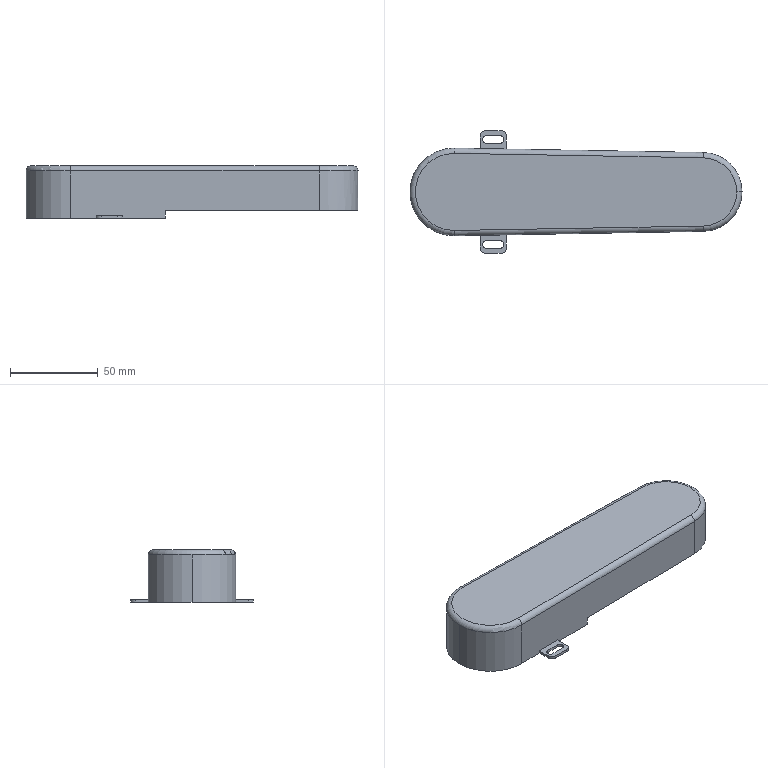Part | SolidWorks | features ICE 3, Extrusion 1, Fillet 1, MirrorPattern 1, Shell 1 | 1 solid | 48 faces | box 189.5 x 70 x 30 mm | volume 29758 mm3 | plane 22 | cylinder 20 | torus 6 | commonest cylinder face diameters 6 x8 4.2 x6 47 x2 50 x2 42 x1 45 x1
STEP:
#1=CARTESIAN_POINT('',(164.5,0.,27.));
#2=VERTEX_POINT('',#1);
#3=CARTESIAN_POINT('',(142.396,-22.497,27.));
#4=VERTEX_POINT('',#3);
#5=CARTESIAN_POINT('',(142.,0.,27.));
#6=DIRECTION('',(0.,0.,-1.));
#7=DIRECTION('',(1.,0.,0.));
#8=AXIS2_PLACEMENT_3D('',#5,#6,#7);
#9=CIRCLE('',#8,22.5);
#10=EDGE_CURVE('',#2,#4,#9,.T.);
#11=ORIENTED_EDGE('',*,*,#10,.F.);
#12=CARTESIAN_POINT('',(161.5,0.,30.));
#13=VERTEX_POINT('',#12);
#14=CARTESIAN_POINT('',(161.5,0.,27.));
#15=DIRECTION('',(0.,-1.,0.));
#16=DIRECTION('',(0.,0.,-1.));
#17=AXIS2_PLACEMENT_3D('',#14,#15,#16);
#18=CIRCLE('',#17,3.);
#19=EDGE_CURVE('',#2,#13,#18,.T.);
#20=ORIENTED_EDGE('',*,*,#19,.T.);
#21=CARTESIAN_POINT('',(142.343,-19.497,30.));
#22=VERTEX_POINT('',#21);
#23=CARTESIAN_POINT('',(142.,0.,30.));
#24=DIRECTION('',(0.,0.,1.));
#25=DIRECTION('',(1.,0.,0.));
#26=AXIS2_PLACEMENT_3D('',#23,#24,#25);
#27=CIRCLE('',#26,19.5);
#28=EDGE_CURVE('',#22,#13,#27,.T.);
#29=ORIENTED_EDGE('',*,*,#28,.F.);
#30=CARTESIAN_POINT('',(142.343,-19.497,27.));
#31=DIRECTION('',(-0.9998,-0.01761,0.));
#32=DIRECTION('',(0.01761,-0.9998,0.));
#33=AXIS2_PLACEMENT_3D('',#30,#31,#32);
#34=CIRCLE('',#33,3.);
#35=EDGE_CURVE('',#4,#22,#34,.T.);
#36=ORIENTED_EDGE('',*,*,#35,.F.);
#37=EDGE_LOOP('',(#11,#20,#29,#36));
#38=FACE_OUTER_BOUND('',#37,.T.);
#39=CARTESIAN_POINT('',(142.,0.,27.));
#40=DIRECTION('',(0.,0.,1.));
#41=DIRECTION('',(1.,0.,0.));
#42=AXIS2_PLACEMENT_3D('',#39,#40,#41);
#43=TOROIDAL_SURFACE('',#42,19.5,3.);
#44=ADVANCED_FACE('',(#38),#43,.T.);
#45=CARTESIAN_POINT('',(163.,0.,25.5));
#46=VERTEX_POINT('',#45);
#47=CARTESIAN_POINT('',(142.37,20.997,25.5));
#48=VERTEX_POINT('',#47);
#49=CARTESIAN_POINT('',(142.,0.,25.5));
#50=DIRECTION('',(0.,0.,1.));
#51=DIRECTION('',(1.,0.,0.));
#52=AXIS2_PLACEMENT_3D('',#49,#50,#51);
#53=CIRCLE('',#52,21.);
#54=EDGE_CURVE('',#46,#48,#53,.T.);
#55=ORIENTED_EDGE('',*,*,#54,.F.);
#56=CARTESIAN_POINT('',(160.,0.,28.5));
#57=VERTEX_POINT('',#56);
#58=CARTESIAN_POINT('',(160.,0.,25.5));
#59=DIRECTION('',(0.,-1.,0.));
#60=DIRECTION('',(0.,0.,-1.));
#61=AXIS2_PLACEMENT_3D('',#58,#59,#60);
#62=CIRCLE('',#61,3.);
#63=EDGE_CURVE('',#46,#57,#62,.T.);
#64=ORIENTED_EDGE('',*,*,#63,.T.);
#65=CARTESIAN_POINT('',(142.317,17.997,28.5));
#66=VERTEX_POINT('',#65);
#67=CARTESIAN_POINT('',(142.,0.,28.5));
#68=DIRECTION('',(0.,0.,-1.));
#69=DIRECTION('',(1.,0.,0.));
#70=AXIS2_PLACEMENT_3D('',#67,#68,#69);
#71=CIRCLE('',#70,18.);
#72=EDGE_CURVE('',#66,#57,#71,.T.);
#73=ORIENTED_EDGE('',*,*,#72,.F.);
#74=CARTESIAN_POINT('',(142.317,17.997,25.5));
#75=DIRECTION('',(-0.9998,0.01761,0.));
#76=DIRECTION('',(-0.01761,-0.9998,0.));
#77=AXIS2_PLACEMENT_3D('',#74,#75,#76);
#78=CIRCLE('',#77,3.);
#79=EDGE_CURVE('',#66,#48,#78,.T.);
#80=ORIENTED_EDGE('',*,*,#79,.T.);
#81=EDGE_LOOP('',(#55,#64,#73,#80));
#82=FACE_OUTER_BOUND('',#81,.T.);
#83=CARTESIAN_POINT('',(142.,0.,25.5));
#84=DIRECTION('',(0.,0.,1.));
#85=DIRECTION('',(1.,0.,0.));
#86=AXIS2_PLACEMENT_3D('',#83,#84,#85);
#87=TOROIDAL_SURFACE('',#86,18.,3.);
#88=ADVANCED_FACE('',(#82),#87,.F.);
#89=CARTESIAN_POINT('',(28.6,-30.,0.));
#90=VERTEX_POINT('',#89);
#91=CARTESIAN_POINT('',(26.5,-27.9,0.));
#92=VERTEX_POINT('',#91);
#93=CARTESIAN_POINT('',(26.5,-30.,0.));
#94=DIRECTION('',(0.,0.,1.));
#95=DIRECTION('',(1.,0.,0.));
#96=AXIS2_PLACEMENT_3D('',#93,#94,#95);
#97=CIRCLE('',#96,2.1);
#98=EDGE_CURVE('',#90,#92,#97,.T.);
#99=ORIENTED_EDGE('',*,*,#98,.F.);
#100=CARTESIAN_POINT('',(28.6,-30.,1.5));
#101=VERTEX_POINT('',#100);
#102=CARTESIAN_POINT('',(28.6,-30.,-12.903));
#103=DIRECTION('',(0.,0.,1.));
#104=VECTOR('',#103,1000.);
#105=LINE('',#102,#104);
#106=EDGE_CURVE('',#90,#101,#105,.T.);
#107=ORIENTED_EDGE('',*,*,#106,.T.);
#108=CARTESIAN_POINT('',(26.5,-27.9,1.5));
#109=VERTEX_POINT('',#108);
#110=CARTESIAN_POINT('',(26.5,-30.,1.5));
#111=DIRECTION('',(0.,0.,-1.));
#112=DIRECTION('',(1.,0.,0.));
#113=AXIS2_PLACEMENT_3D('',#110,#111,#112);
#114=CIRCLE('',#113,2.1);
#115=EDGE_CURVE('',#109,#101,#114,.T.);
#116=ORIENTED_EDGE('',*,*,#115,.F.);
#117=CARTESIAN_POINT('',(26.5,-27.9,-12.903));
#118=DIRECTION('',(0.,0.,1.));
#119=VECTOR('',#118,1000.);
#120=LINE('',#117,#119);
#121=EDGE_CURVE('',#92,#109,#120,.T.);
#122=ORIENTED_EDGE('',*,*,#121,.F.);
#123=EDGE_LOOP('',(#99,#107,#116,#122));
#124=FACE_OUTER_BOUND('',#123,.T.);
#125=CARTESIAN_POINT('',(26.5,-30.,-12.903));
#126=DIRECTION('',(0.,0.,1.));
#127=DIRECTION('',(1.,0.,0.));
#128=AXIS2_PLACEMENT_3D('',#125,#126,#127);
#129=CYLINDRICAL_SURFACE('',#128,2.1);
#130=ADVANCED_FACE('',(#124),#129,.F.);
#131=CARTESIAN_POINT('',(26.5,32.1,0.));
#132=VERTEX_POINT('',#131);
#133=CARTESIAN_POINT('',(28.6,30.,0.));
#134=VERTEX_POINT('',#133);
#135=CARTESIAN_POINT('',(26.5,30.,0.));
#136=DIRECTION('',(0.,0.,-1.));
#137=DIRECTION('',(1.,0.,0.));
#138=AXIS2_PLACEMENT_3D('',#135,#136,#137);
#139=CIRCLE('',#138,2.1);
#140=EDGE_CURVE('',#132,#134,#139,.T.);
#141=ORIENTED_EDGE('',*,*,#140,.T.);
#142=CARTESIAN_POINT('',(28.6,30.,1.5));
#143=VERTEX_POINT('',#142);
#144=CARTESIAN_POINT('',(28.6,30.,-12.903));
#145=DIRECTION('',(0.,0.,1.));
#146=VECTOR('',#145,1000.);
#147=LINE('',#144,#146);
#148=EDGE_CURVE('',#134,#143,#147,.T.);
#149=ORIENTED_EDGE('',*,*,#148,.T.);
#150=CARTESIAN_POINT('',(26.5,32.1,1.5));
#151=VERTEX_POINT('',#150);
#152=CARTESIAN_POINT('',(26.5,30.,1.5));
#153=DIRECTION('',(0.,0.,1.));
#154=DIRECTION('',(1.,0.,0.));
#155=AXIS2_PLACEMENT_3D('',#152,#153,#154);
#156=CIRCLE('',#155,2.1);
#157=EDGE_CURVE('',#143,#151,#156,.T.);
#158=ORIENTED_EDGE('',*,*,#157,.T.);
#159=CARTESIAN_POINT('',(26.5,32.1,-12.903));
#160=DIRECTION('',(0.,0.,1.));
#161=VECTOR('',#160,1000.);
#162=LINE('',#159,#161);
#163=EDGE_CURVE('',#132,#151,#162,.T.);
#164=ORIENTED_EDGE('',*,*,#163,.F.);
#165=EDGE_LOOP('',(#141,#149,#158,#164));
#166=FACE_OUTER_BOUND('',#165,.T.);
#167=CARTESIAN_POINT('',(26.5,30.,-12.903));
#168=DIRECTION('',(0.,0.,1.));
#169=DIRECTION('',(1.,0.,0.));
#170=AXIS2_PLACEMENT_3D('',#167,#168,#169);
#171=CYLINDRICAL_SURFACE('',#170,2.1);
#172=ADVANCED_FACE('',(#166),#171,.F.);
#173=CARTESIAN_POINT('',(0.4137,23.496,25.5));
#174=VERTEX_POINT('',#173);
#175=CARTESIAN_POINT('',(-23.5,0.,25.5));
#176=VERTEX_POINT('',#175);
#177=CARTESIAN_POINT('',(0.,0.,25.5));
#178=DIRECTION('',(0.,0.,1.));
#179=DIRECTION('',(1.,0.,0.));
#180=AXIS2_PLACEMENT_3D('',#177,#178,#179);
#181=CIRCLE('',#180,23.5);
#182=EDGE_CURVE('',#174,#176,#181,.T.);
#183=ORIENTED_EDGE('',*,*,#182,.T.);
#184=CARTESIAN_POINT('',(-23.5,0.,0.));
#185=VERTEX_POINT('',#184);
#186=CARTESIAN_POINT('',(-23.5,0.,30.));
#187=DIRECTION('',(0.,0.,-1.));
#188=VECTOR('',#187,1000.);
#189=LINE('',#186,#188);
#190=EDGE_CURVE('',#176,#185,#189,.T.);
#191=ORIENTED_EDGE('',*,*,#190,.T.);
#192=CARTESIAN_POINT('',(0.4137,23.496,0.));
#193=VERTEX_POINT('',#192);
#194=CARTESIAN_POINT('',(0.,0.,0.));
#195=DIRECTION('',(0.,0.,1.));
#196=DIRECTION('',(1.,0.,0.));
#197=AXIS2_PLACEMENT_3D('',#194,#195,#196);
#198=CIRCLE('',#197,23.5);
#199=EDGE_CURVE('',#193,#185,#198,.T.);
#200=ORIENTED_EDGE('',*,*,#199,.F.);
#201=CARTESIAN_POINT('',(0.4137,23.496,30.));
#202=DIRECTION('',(0.,0.,-1.));
#203=VECTOR('',#202,1000.);
#204=LINE('',#201,#203);
#205=EDGE_CURVE('',#174,#193,#204,.T.);
#206=ORIENTED_EDGE('',*,*,#205,.F.);
#207=EDGE_LOOP('',(#183,#191,#200,#206));
#208=FACE_OUTER_BOUND('',#207,.T.);
#209=CARTESIAN_POINT('',(0.,0.,30.));
#210=DIRECTION('',(0.,0.,-1.));
#211=DIRECTION('',(-1.,0.,0.));
#212=AXIS2_PLACEMENT_3D('',#209,#210,#211);
#213=CYLINDRICAL_SURFACE('',#212,23.5);
#214=ADVANCED_FACE('',(#208),#213,.F.);
#215=CARTESIAN_POINT('',(0.4401,-24.996,27.));
#216=VERTEX_POINT('',#215);
#217=CARTESIAN_POINT('',(-25.,0.,27.));
#218=VERTEX_POINT('',#217);
#219=CARTESIAN_POINT('',(0.,0.,27.));
#220=DIRECTION('',(0.,0.,-1.));
#221=DIRECTION('',(1.,0.,0.));
#222=AXIS2_PLACEMENT_3D('',#219,#220,#221);
#223=CIRCLE('',#222,25.);
#224=EDGE_CURVE('',#216,#218,#223,.T.);
#225=ORIENTED_EDGE('',*,*,#224,.T.);
#226=CARTESIAN_POINT('',(-25.,0.,0.));
#227=VERTEX_POINT('',#226);
#228=CARTESIAN_POINT('',(-25.,0.,30.));
#229=DIRECTION('',(0.,0.,-1.));
#230=VECTOR('',#229,1000.);
#231=LINE('',#228,#230);
#232=EDGE_CURVE('',#218,#227,#231,.T.);
#233=ORIENTED_EDGE('',*,*,#232,.T.);
#234=CARTESIAN_POINT('',(0.4401,-24.996,0.));
#235=VERTEX_POINT('',#234);
#236=CARTESIAN_POINT('',(0.,0.,0.));
#237=DIRECTION('',(0.,0.,1.));
#238=DIRECTION('',(1.,0.,0.));
#239=AXIS2_PLACEMENT_3D('',#236,#237,#238);
#240=CIRCLE('',#239,25.);
#241=EDGE_CURVE('',#227,#235,#240,.T.);
#242=ORIENTED_EDGE('',*,*,#241,.T.);
#243=CARTESIAN_POINT('',(0.4401,-24.996,30.));
#244=DIRECTION('',(0.,0.,-1.));
#245=VECTOR('',#244,1000.);
#246=LINE('',#243,#245);
#247=EDGE_CURVE('',#216,#235,#246,.T.);
#248=ORIENTED_EDGE('',*,*,#247,.F.);
#249=EDGE_LOOP('',(#225,#233,#242,#248));
#250=FACE_OUTER_BOUND('',#249,.T.);
#251=CARTESIAN_POINT('',(0.,0.,30.));
#252=DIRECTION('',(0.,0.,-1.));
#253=DIRECTION('',(-1.,0.,0.));
#254=AXIS2_PLACEMENT_3D('',#251,#252,#253);
#255=CYLINDRICAL_SURFACE('',#254,25.);
#256=ADVANCED_FACE('',(#250),#255,.T.);
#257=CARTESIAN_POINT('',(30.,-24.476,0.));
#258=VERTEX_POINT('',#257);
#259=CARTESIAN_POINT('',(54.5,-24.044,0.));
#260=VERTEX_POINT('',#259);
#261=CARTESIAN_POINT('',(0.4401,-24.996,0.));
#262=DIRECTION('',(0.9998,0.01761,0.));
#263=VECTOR('',#262,1000.);
#264=LINE('',#261,#263);
#265=EDGE_CURVE('',#258,#260,#264,.T.);
#266=ORIENTED_EDGE('',*,*,#265,.T.);
#267=CARTESIAN_POINT('',(54.5,-24.044,4.5));
#268=VERTEX_POINT('',#267);
#269=CARTESIAN_POINT('',(54.5,-24.044,30.));
#270=DIRECTION('',(0.,0.,1.));
#271=VECTOR('',#270,1000.);
#272=LINE('',#269,#271);
#273=EDGE_CURVE('',#260,#268,#272,.T.);
#274=ORIENTED_EDGE('',*,*,#273,.T.);
#275=CARTESIAN_POINT('',(142.396,-22.497,4.5));
#276=VERTEX_POINT('',#275);
#277=CARTESIAN_POINT('',(0.4401,-24.996,4.5));
#278=DIRECTION('',(0.9998,0.01761,0.));
#279=VECTOR('',#278,1000.);
#280=LINE('',#277,#279);
#281=EDGE_CURVE('',#268,#276,#280,.T.);
#282=ORIENTED_EDGE('',*,*,#281,.T.);
#283=CARTESIAN_POINT('',(142.396,-22.497,30.));
#284=DIRECTION('',(0.,0.,-1.));
#285=VECTOR('',#284,1000.);
#286=LINE('',#283,#285);
#287=EDGE_CURVE('',#4,#276,#286,.T.);
#288=ORIENTED_EDGE('',*,*,#287,.F.);
#289=CARTESIAN_POINT('',(0.4401,-24.996,27.));
#290=DIRECTION('',(-0.9998,-0.01761,0.));
#291=VECTOR('',#290,1000.);
#292=LINE('',#289,#291);
#293=EDGE_CURVE('',#4,#216,#292,.T.);
#294=ORIENTED_EDGE('',*,*,#293,.T.);
#295=ORIENTED_EDGE('',*,*,#247,.T.);
#296=CARTESIAN_POINT('',(15.,-24.74,0.));
#297=VERTEX_POINT('',#296);
#298=CARTESIAN_POINT('',(0.4401,-24.996,0.));
#299=DIRECTION('',(0.9998,0.01761,0.));
#300=VECTOR('',#299,1000.);
#301=LINE('',#298,#300);
#302=EDGE_CURVE('',#235,#297,#301,.T.);
#303=ORIENTED_EDGE('',*,*,#302,.T.);
#304=CARTESIAN_POINT('',(15.,-24.74,1.5));
#305=VERTEX_POINT('',#304);
#306=CARTESIAN_POINT('',(15.,-24.74,1.5));
#307=DIRECTION('',(0.,0.,-1.));
#308=VECTOR('',#307,1000.);
#309=LINE('',#306,#308);
#310=EDGE_CURVE('',#305,#297,#309,.T.);
#311=ORIENTED_EDGE('',*,*,#310,.F.);
#312=CARTESIAN_POINT('',(30.,-24.476,1.5));
#313=VERTEX_POINT('',#312);
#314=CARTESIAN_POINT('',(15.,-24.74,1.5));
#315=DIRECTION('',(-0.9998,-0.01761,0.));
#316=VECTOR('',#315,1000.);
#317=LINE('',#314,#316);
#318=EDGE_CURVE('',#313,#305,#317,.T.);
#319=ORIENTED_EDGE('',*,*,#318,.F.);
#320=CARTESIAN_POINT('',(30.,-24.476,1.5));
#321=DIRECTION('',(0.,0.,-1.));
#322=VECTOR('',#321,1000.);
#323=LINE('',#320,#322);
#324=EDGE_CURVE('',#313,#258,#323,.T.);
#325=ORIENTED_EDGE('',*,*,#324,.T.);
#326=EDGE_LOOP('',(#266,#274,#282,#288,#294,#295,#303,#311,#319,#325));
#327=FACE_OUTER_BOUND('',#326,.T.);
#328=CARTESIAN_POINT('',(0.4401,-24.996,30.));
#329=DIRECTION('',(-0.01761,0.9998,0.));
#330=DIRECTION('',(-0.9998,-0.01761,0.));
#331=AXIS2_PLACEMENT_3D('',#328,#329,#330);
#332=PLANE('',#331);
#333=ADVANCED_FACE('',(#327),#332,.F.);
#334=ORIENTED_EDGE('',*,*,#232,.F.);
#335=CARTESIAN_POINT('',(0.4401,24.996,27.));
#336=VERTEX_POINT('',#335);
#337=CARTESIAN_POINT('',(0.,0.,27.));
#338=DIRECTION('',(0.,0.,-1.));
#339=DIRECTION('',(1.,0.,0.));
#340=AXIS2_PLACEMENT_3D('',#337,#338,#339);
#341=CIRCLE('',#340,25.);
#342=EDGE_CURVE('',#218,#336,#341,.T.);
#343=ORIENTED_EDGE('',*,*,#342,.T.);
#344=CARTESIAN_POINT('',(0.4401,24.996,0.));
#345=VERTEX_POINT('',#344);
#346=CARTESIAN_POINT('',(0.4401,24.996,30.));
#347=DIRECTION('',(0.,0.,-1.));
#348=VECTOR('',#347,1000.);
#349=LINE('',#346,#348);
#350=EDGE_CURVE('',#336,#345,#349,.T.);
#351=ORIENTED_EDGE('',*,*,#350,.T.);
#352=CARTESIAN_POINT('',(0.,0.,0.));
#353=DIRECTION('',(0.,0.,1.));
#354=DIRECTION('',(1.,0.,0.));
#355=AXIS2_PLACEMENT_3D('',#352,#353,#354);
#356=CIRCLE('',#355,25.);
#357=EDGE_CURVE('',#345,#227,#356,.T.);
#358=ORIENTED_EDGE('',*,*,#357,.T.);
#359=EDGE_LOOP('',(#334,#343,#351,#358));
#360=FACE_OUTER_BOUND('',#359,.T.);
#361=CARTESIAN_POINT('',(0.,0.,30.));
#362=DIRECTION('',(0.,0.,-1.));
#363=DIRECTION('',(-1.,0.,0.));
#364=AXIS2_PLACEMENT_3D('',#361,#362,#363);
#365=CYLINDRICAL_SURFACE('',#364,25.);
#366=ADVANCED_FACE('',(#360),#365,.T.);
#367=CARTESIAN_POINT('',(142.396,22.497,4.5));
#368=VERTEX_POINT('',#367);
#369=CARTESIAN_POINT('',(142.,0.,4.5));
#370=DIRECTION('',(0.,0.,1.));
#371=DIRECTION('',(1.,0.,0.));
#372=AXIS2_PLACEMENT_3D('',#369,#370,#371);
#373=CIRCLE('',#372,22.5);
#374=EDGE_CURVE('',#276,#368,#373,.T.);
#375=ORIENTED_EDGE('',*,*,#374,.T.);
#376=CARTESIAN_POINT('',(142.396,22.497,27.));
#377=VERTEX_POINT('',#376);
#378=CARTESIAN_POINT('',(142.396,22.497,30.));
#379=DIRECTION('',(0.,0.,-1.));
#380=VECTOR('',#379,1000.);
#381=LINE('',#378,#380);
#382=EDGE_CURVE('',#377,#368,#381,.T.);
#383=ORIENTED_EDGE('',*,*,#382,.F.);
#384=CARTESIAN_POINT('',(142.,0.,27.));
#385=DIRECTION('',(0.,0.,-1.));
#386=DIRECTION('',(1.,0.,0.));
#387=AXIS2_PLACEMENT_3D('',#384,#385,#386);
#388=CIRCLE('',#387,22.5);
#389=EDGE_CURVE('',#377,#2,#388,.T.);
#390=ORIENTED_EDGE('',*,*,#389,.T.);
#391=ORIENTED_EDGE('',*,*,#10,.T.);
#392=ORIENTED_EDGE('',*,*,#287,.T.);
#393=EDGE_LOOP('',(#375,#383,#390,#391,#392));
#394=FACE_OUTER_BOUND('',#393,.T.);
#395=CARTESIAN_POINT('',(142.,0.,30.));
#396=DIRECTION('',(0.,0.,-1.));
#397=DIRECTION('',(-1.,0.,0.));
#398=AXIS2_PLACEMENT_3D('',#395,#396,#397);
#399=CYLINDRICAL_SURFACE('',#398,22.5);
#400=ADVANCED_FACE('',(#394),#399,.T.);
#401=CARTESIAN_POINT('',(54.5,24.044,4.5));
#402=VERTEX_POINT('',#401);
#403=CARTESIAN_POINT('',(0.4401,24.996,4.5));
#404=DIRECTION('',(-0.9998,0.01761,0.));
#405=VECTOR('',#404,1000.);
#406=LINE('',#403,#405);
#407=EDGE_CURVE('',#368,#402,#406,.T.);
#408=ORIENTED_EDGE('',*,*,#407,.T.);
#409=CARTESIAN_POINT('',(54.5,24.044,0.));
#410=VERTEX_POINT('',#409);
#411=CARTESIAN_POINT('',(54.5,24.044,30.));
#412=DIRECTION('',(0.,0.,-1.));
#413=VECTOR('',#412,1000.);
#414=LINE('',#411,#413);
#415=EDGE_CURVE('',#402,#410,#414,.T.);
#416=ORIENTED_EDGE('',*,*,#415,.T.);
#417=CARTESIAN_POINT('',(30.,24.476,0.));
#418=VERTEX_POINT('',#417);
#419=CARTESIAN_POINT('',(0.4401,24.996,0.));
#420=DIRECTION('',(-0.9998,0.01761,0.));
#421=VECTOR('',#420,1000.);
#422=LINE('',#419,#421);
#423=EDGE_CURVE('',#410,#418,#422,.T.);
#424=ORIENTED_EDGE('',*,*,#423,.T.);
#425=CARTESIAN_POINT('',(30.,24.476,1.5));
#426=VERTEX_POINT('',#425);
#427=CARTESIAN_POINT('',(30.,24.476,1.5));
#428=DIRECTION('',(0.,0.,-1.));
#429=VECTOR('',#428,1000.);
#430=LINE('',#427,#429);
#431=EDGE_CURVE('',#426,#418,#430,.T.);
#432=ORIENTED_EDGE('',*,*,#431,.F.);
#433=CARTESIAN_POINT('',(15.,24.74,1.5));
#434=VERTEX_POINT('',#433);
#435=CARTESIAN_POINT('',(15.,24.74,1.5));
#436=DIRECTION('',(-0.9998,0.01761,0.));
#437=VECTOR('',#436,1000.);
#438=LINE('',#435,#437);
#439=EDGE_CURVE('',#426,#434,#438,.T.);
#440=ORIENTED_EDGE('',*,*,#439,.T.);
#441=CARTESIAN_POINT('',(15.,24.74,0.));
#442=VERTEX_POINT('',#441);
#443=CARTESIAN_POINT('',(15.,24.74,1.5));
#444=DIRECTION('',(0.,0.,-1.));
#445=VECTOR('',#444,1000.);
#446=LINE('',#443,#445);
#447=EDGE_CURVE('',#434,#442,#446,.T.);
#448=ORIENTED_EDGE('',*,*,#447,.T.);
#449=CARTESIAN_POINT('',(0.4401,24.996,0.));
#450=DIRECTION('',(-0.9998,0.01761,0.));
#451=VECTOR('',#450,1000.);
#452=LINE('',#449,#451);
#453=EDGE_CURVE('',#442,#345,#452,.T.);
#454=ORIENTED_EDGE('',*,*,#453,.T.);
#455=ORIENTED_EDGE('',*,*,#350,.F.);
#456=CARTESIAN_POINT('',(142.396,22.497,27.));
#457=DIRECTION('',(0.9998,-0.01761,0.));
#458=VECTOR('',#457,1000.);
#459=LINE('',#456,#458);
#460=EDGE_CURVE('',#336,#377,#459,.T.);
#461=ORIENTED_EDGE('',*,*,#460,.T.);
#462=ORIENTED_EDGE('',*,*,#382,.T.);
#463=EDGE_LOOP('',(#408,#416,#424,#432,#440,#448,#454,#455,#461,#462));
#464=FACE_OUTER_BOUND('',#463,.T.);
#465=CARTESIAN_POINT('',(0.4401,24.996,30.));
#466=DIRECTION('',(-0.01761,-0.9998,0.));
#467=DIRECTION('',(0.9998,-0.01761,0.));
#468=AXIS2_PLACEMENT_3D('',#465,#466,#467);
#469=PLANE('',#468);
#470=ADVANCED_FACE('',(#464),#469,.F.);
#471=CARTESIAN_POINT('',(142.343,19.497,30.));
#472=VERTEX_POINT('',#471);
#473=CARTESIAN_POINT('',(0.3873,21.997,30.));
#474=VERTEX_POINT('',#473);
#475=CARTESIAN_POINT('',(0.3873,21.997,30.));
#476=DIRECTION('',(-0.9998,0.01761,0.));
#477=VECTOR('',#476,1000.);
#478=LINE('',#475,#477);
#479=EDGE_CURVE('',#472,#474,#478,.T.);
#480=ORIENTED_EDGE('',*,*,#479,.T.);
#481=CARTESIAN_POINT('',(0.3873,-21.997,30.));
#482=VERTEX_POINT('',#481);
#483=CARTESIAN_POINT('',(0.,0.,30.));
#484=DIRECTION('',(0.,0.,1.));
#485=DIRECTION('',(1.,0.,0.));
#486=AXIS2_PLACEMENT_3D('',#483,#484,#485);
#487=CIRCLE('',#486,22.);
#488=EDGE_CURVE('',#474,#482,#487,.T.);
#489=ORIENTED_EDGE('',*,*,#488,.T.);
#490=CARTESIAN_POINT('',(142.343,-19.497,30.));
#491=DIRECTION('',(0.9998,0.01761,0.));
#492=VECTOR('',#491,1000.);
#493=LINE('',#490,#492);
#494=EDGE_CURVE('',#482,#22,#493,.T.);
#495=ORIENTED_EDGE('',*,*,#494,.T.);
#496=ORIENTED_EDGE('',*,*,#28,.T.);
#497=CARTESIAN_POINT('',(142.,0.,30.));
#498=DIRECTION('',(0.,0.,1.));
#499=DIRECTION('',(1.,0.,0.));
#500=AXIS2_PLACEMENT_3D('',#497,#498,#499);
#501=CIRCLE('',#500,19.5);
#502=EDGE_CURVE('',#13,#472,#501,.T.);
#503=ORIENTED_EDGE('',*,*,#502,.T.);
#504=EDGE_LOOP('',(#480,#489,#495,#496,#503));
#505=FACE_OUTER_BOUND('',#504,.T.);
#506=CARTESIAN_POINT('',(0.,0.,30.));
#507=DIRECTION('',(0.,0.,1.));
#508=DIRECTION('',(1.,0.,0.));
#509=AXIS2_PLACEMENT_3D('',#506,#507,#508);
#510=PLANE('',#509);
#511=ADVANCED_FACE('',(#505),#510,.T.);
#512=CARTESIAN_POINT('',(18.5,-27.9,0.));
#513=VERTEX_POINT('',#512);
#514=CARTESIAN_POINT('',(26.5,-27.9,0.));
#515=DIRECTION('',(-1.,0.,0.));
#516=VECTOR('',#515,1000.);
#517=LINE('',#514,#516);
#518=EDGE_CURVE('',#92,#513,#517,.T.);
#519=ORIENTED_EDGE('',*,*,#518,.T.);
#520=CARTESIAN_POINT('',(18.5,-32.1,0.));
#521=VERTEX_POINT('',#520);
#522=CARTESIAN_POINT('',(18.5,-30.,0.));
#523=DIRECTION('',(0.,0.,1.));
#524=DIRECTION('',(1.,0.,0.));
#525=AXIS2_PLACEMENT_3D('',#522,#523,#524);
#526=CIRCLE('',#525,2.1);
#527=EDGE_CURVE('',#513,#521,#526,.T.);
#528=ORIENTED_EDGE('',*,*,#527,.T.);
#529=CARTESIAN_POINT('',(26.5,-32.1,0.));
#530=VERTEX_POINT('',#529);
#531=CARTESIAN_POINT('',(26.5,-32.1,0.));
#532=DIRECTION('',(1.,0.,0.));
#533=VECTOR('',#532,1000.);
#534=LINE('',#531,#533);
#535=EDGE_CURVE('',#521,#530,#534,.T.);
#536=ORIENTED_EDGE('',*,*,#535,.T.);
#537=CARTESIAN_POINT('',(26.5,-30.,0.));
#538=DIRECTION('',(0.,0.,1.));
#539=DIRECTION('',(1.,0.,0.));
#540=AXIS2_PLACEMENT_3D('',#537,#538,#539);
#541=CIRCLE('',#540,2.1);
#542=EDGE_CURVE('',#530,#90,#541,.T.);
#543=ORIENTED_EDGE('',*,*,#542,.T.);
#544=ORIENTED_EDGE('',*,*,#98,.T.);
#545=EDGE_LOOP('',(#519,#528,#536,#543,#544));
#546=FACE_BOUND('',#545,.T.);
#547=CARTESIAN_POINT('',(26.5,27.9,0.));
#548=VERTEX_POINT('',#547);
#549=CARTESIAN_POINT('',(18.5,27.9,0.));
#550=VERTEX_POINT('',#549);
#551=CARTESIAN_POINT('',(26.5,27.9,0.));
#552=DIRECTION('',(-1.,0.,0.));
#553=VECTOR('',#552,1000.);
#554=LINE('',#551,#553);
#555=EDGE_CURVE('',#548,#550,#554,.T.);
#556=ORIENTED_EDGE('',*,*,#555,.F.);
#557=CARTESIAN_POINT('',(26.5,30.,0.));
#558=DIRECTION('',(0.,0.,-1.));
#559=DIRECTION('',(1.,0.,0.));
#560=AXIS2_PLACEMENT_3D('',#557,#558,#559);
#561=CIRCLE('',#560,2.1);
#562=EDGE_CURVE('',#134,#548,#561,.T.);
#563=ORIENTED_EDGE('',*,*,#562,.F.);
#564=ORIENTED_EDGE('',*,*,#140,.F.);
#565=CARTESIAN_POINT('',(18.5,32.1,0.));
#566=VERTEX_POINT('',#565);
#567=CARTESIAN_POINT('',(26.5,32.1,0.));
#568=DIRECTION('',(1.,0.,0.));
#569=VECTOR('',#568,1000.);
#570=LINE('',#567,#569);
#571=EDGE_CURVE('',#566,#132,#570,.T.);
#572=ORIENTED_EDGE('',*,*,#571,.F.);
#573=CARTESIAN_POINT('',(18.5,30.,0.));
#574=DIRECTION('',(0.,0.,-1.));
#575=DIRECTION('',(1.,0.,0.));
#576=AXIS2_PLACEMENT_3D('',#573,#574,#575);
#577=CIRCLE('',#576,2.1);
#578=EDGE_CURVE('',#550,#566,#577,.T.);
#579=ORIENTED_EDGE('',*,*,#578,.F.);
#580=EDGE_LOOP('',(#556,#563,#564,#572,#579));
#581=FACE_BOUND('',#580,.T.);
#582=ORIENTED_EDGE('',*,*,#423,.F.);
#583=CARTESIAN_POINT('',(54.5,22.544,0.));
#584=VERTEX_POINT('',#583);
#585=CARTESIAN_POINT('',(54.5,-30.,0.));
#586=DIRECTION('',(0.,1.,0.));
#587=VECTOR('',#586,1000.);
#588=LINE('',#585,#587);
#589=EDGE_CURVE('',#584,#410,#588,.T.);
#590=ORIENTED_EDGE('',*,*,#589,.F.);
#591=CARTESIAN_POINT('',(0.4137,23.496,0.));
#592=DIRECTION('',(-0.9998,0.01761,0.));
#593=VECTOR('',#592,1000.);
#594=LINE('',#591,#593);
#595=EDGE_CURVE('',#584,#193,#594,.T.);
#596=ORIENTED_EDGE('',*,*,#595,.T.);
#597=ORIENTED_EDGE('',*,*,#199,.T.);
#598=CARTESIAN_POINT('',(0.4137,-23.496,0.));
#599=VERTEX_POINT('',#598);
#600=CARTESIAN_POINT('',(0.,0.,0.));
#601=DIRECTION('',(0.,0.,1.));
#602=DIRECTION('',(1.,0.,0.));
#603=AXIS2_PLACEMENT_3D('',#600,#601,#602);
#604=CIRCLE('',#603,23.5);
#605=EDGE_CURVE('',#185,#599,#604,.T.);
#606=ORIENTED_EDGE('',*,*,#605,.T.);
#607=CARTESIAN_POINT('',(54.5,-22.544,0.));
#608=VERTEX_POINT('',#607);
#609=CARTESIAN_POINT('',(0.4137,-23.496,0.));
#610=DIRECTION('',(0.9998,0.01761,0.));
#611=VECTOR('',#610,1000.);
#612=LINE('',#609,#611);
#613=EDGE_CURVE('',#599,#608,#612,.T.);
#614=ORIENTED_EDGE('',*,*,#613,.T.);
#615=CARTESIAN_POINT('',(54.5,-30.,0.));
#616=DIRECTION('',(0.,1.,0.));
#617=VECTOR('',#616,1000.);
#618=LINE('',#615,#617);
#619=EDGE_CURVE('',#260,#608,#618,.T.);
#620=ORIENTED_EDGE('',*,*,#619,.F.);
#621=ORIENTED_EDGE('',*,*,#265,.F.);
#622=CARTESIAN_POINT('',(30.,-32.,0.));
#623=VERTEX_POINT('',#622);
#624=CARTESIAN_POINT('',(30.,-24.476,0.));
#625=DIRECTION('',(0.,1.,0.));
#626=VECTOR('',#625,1000.);
#627=LINE('',#624,#626);
#628=EDGE_CURVE('',#623,#258,#627,.T.);
#629=ORIENTED_EDGE('',*,*,#628,.F.);
#630=CARTESIAN_POINT('',(27.,-35.,0.));
#631=VERTEX_POINT('',#630);
#632=CARTESIAN_POINT('',(27.,-32.,0.));
#633=DIRECTION('',(0.,0.,-1.));
#634=DIRECTION('',(1.,0.,0.));
#635=AXIS2_PLACEMENT_3D('',#632,#633,#634);
#636=CIRCLE('',#635,3.);
#637=EDGE_CURVE('',#623,#631,#636,.T.);
#638=ORIENTED_EDGE('',*,*,#637,.T.);
#639=CARTESIAN_POINT('',(18.,-35.,0.));
#640=VERTEX_POINT('',#639);
#641=CARTESIAN_POINT('',(30.,-35.,0.));
#642=DIRECTION('',(1.,0.,0.));
#643=VECTOR('',#642,1000.);
#644=LINE('',#641,#643);
#645=EDGE_CURVE('',#640,#631,#644,.T.);
#646=ORIENTED_EDGE('',*,*,#645,.F.);
#647=CARTESIAN_POINT('',(15.,-32.,0.));
#648=VERTEX_POINT('',#647);
#649=CARTESIAN_POINT('',(18.,-32.,0.));
#650=DIRECTION('',(0.,0.,-1.));
#651=DIRECTION('',(1.,0.,0.));
#652=AXIS2_PLACEMENT_3D('',#649,#650,#651);
#653=CIRCLE('',#652,3.);
#654=EDGE_CURVE('',#640,#648,#653,.T.);
#655=ORIENTED_EDGE('',*,*,#654,.T.);
#656=CARTESIAN_POINT('',(15.,-35.,0.));
#657=DIRECTION('',(0.,-1.,0.));
#658=VECTOR('',#657,1000.);
#659=LINE('',#656,#658);
#660=EDGE_CURVE('',#297,#648,#659,.T.);
#661=ORIENTED_EDGE('',*,*,#660,.F.);
#662=ORIENTED_EDGE('',*,*,#302,.F.);
#663=ORIENTED_EDGE('',*,*,#241,.F.);
#664=ORIENTED_EDGE('',*,*,#357,.F.);
#665=ORIENTED_EDGE('',*,*,#453,.F.);
#666=CARTESIAN_POINT('',(15.,32.,0.));
#667=VERTEX_POINT('',#666);
#668=CARTESIAN_POINT('',(15.,35.,0.));
#669=DIRECTION('',(0.,1.,0.));
#670=VECTOR('',#669,1000.);
#671=LINE('',#668,#670);
#672=EDGE_CURVE('',#442,#667,#671,.T.);
#673=ORIENTED_EDGE('',*,*,#672,.T.);
#674=CARTESIAN_POINT('',(18.,35.,0.));
#675=VERTEX_POINT('',#674);
#676=CARTESIAN_POINT('',(18.,32.,0.));
#677=DIRECTION('',(0.,0.,-1.));
#678=DIRECTION('',(1.,0.,0.));
#679=AXIS2_PLACEMENT_3D('',#676,#677,#678);
#680=CIRCLE('',#679,3.);
#681=EDGE_CURVE('',#667,#675,#680,.T.);
#682=ORIENTED_EDGE('',*,*,#681,.T.);
#683=CARTESIAN_POINT('',(27.,35.,0.));
#684=VERTEX_POINT('',#683);
#685=CARTESIAN_POINT('',(30.,35.,0.));
#686=DIRECTION('',(1.,0.,0.));
#687=VECTOR('',#686,1000.);
#688=LINE('',#685,#687);
#689=EDGE_CURVE('',#675,#684,#688,.T.);
#690=ORIENTED_EDGE('',*,*,#689,.T.);
#691=CARTESIAN_POINT('',(30.,32.,0.));
#692=VERTEX_POINT('',#691);
#693=CARTESIAN_POINT('',(27.,32.,0.));
#694=DIRECTION('',(0.,0.,-1.));
#695=DIRECTION('',(1.,0.,0.));
#696=AXIS2_PLACEMENT_3D('',#693,#694,#695);
#697=CIRCLE('',#696,3.);
#698=EDGE_CURVE('',#684,#692,#697,.T.);
#699=ORIENTED_EDGE('',*,*,#698,.T.);
#700=CARTESIAN_POINT('',(30.,24.476,0.));
#701=DIRECTION('',(0.,-1.,0.));
#702=VECTOR('',#701,1000.);
#703=LINE('',#700,#702);
#704=EDGE_CURVE('',#692,#418,#703,.T.);
#705=ORIENTED_EDGE('',*,*,#704,.T.);
#706=EDGE_LOOP('',(#582,#590,#596,#597,#606,#614,#620,#621,#629,#638,#646,#655,#661,#662,#663,#664,#665,#673,#682,#690,#699,#705));
#707=FACE_OUTER_BOUND('',#706,.T.);
#708=CARTESIAN_POINT('',(0.,0.,0.));
#709=DIRECTION('',(0.,0.,1.));
#710=DIRECTION('',(1.,0.,0.));
#711=AXIS2_PLACEMENT_3D('',#708,#709,#710);
#712=PLANE('',#711);
#713=ADVANCED_FACE('',(#546,#581,#707),#712,.F.);
#714=ORIENTED_EDGE('',*,*,#190,.F.);
#715=CARTESIAN_POINT('',(0.4137,-23.496,25.5));
#716=VERTEX_POINT('',#715);
#717=CARTESIAN_POINT('',(0.,0.,25.5));
#718=DIRECTION('',(0.,0.,1.));
#719=DIRECTION('',(1.,0.,0.));
#720=AXIS2_PLACEMENT_3D('',#717,#718,#719);
#721=CIRCLE('',#720,23.5);
#722=EDGE_CURVE('',#176,#716,#721,.T.);
#723=ORIENTED_EDGE('',*,*,#722,.T.);
#724=CARTESIAN_POINT('',(0.4137,-23.496,30.));
#725=DIRECTION('',(0.,0.,-1.));
#726=VECTOR('',#725,1000.);
#727=LINE('',#724,#726);
#728=EDGE_CURVE('',#716,#599,#727,.T.);
#729=ORIENTED_EDGE('',*,*,#728,.T.);
#730=ORIENTED_EDGE('',*,*,#605,.F.);
#731=EDGE_LOOP('',(#714,#723,#729,#730));
#732=FACE_OUTER_BOUND('',#731,.T.);
#733=CARTESIAN_POINT('',(0.,0.,30.));
#734=DIRECTION('',(0.,0.,-1.));
#735=DIRECTION('',(-1.,0.,0.));
#736=AXIS2_PLACEMENT_3D('',#733,#734,#735);
#737=CYLINDRICAL_SURFACE('',#736,23.5);
#738=ADVANCED_FACE('',(#732),#737,.F.);
#739=CARTESIAN_POINT('',(54.5,-22.544,4.5));
#740=VERTEX_POINT('',#739);
#741=CARTESIAN_POINT('',(54.5,-22.544,30.));
#742=DIRECTION('',(0.,0.,1.));
#743=VECTOR('',#742,1000.);
#744=LINE('',#741,#743);
#745=EDGE_CURVE('',#608,#740,#744,.T.);
#746=ORIENTED_EDGE('',*,*,#745,.F.);
#747=ORIENTED_EDGE('',*,*,#613,.F.);
#748=ORIENTED_EDGE('',*,*,#728,.F.);
#749=CARTESIAN_POINT('',(142.37,-20.997,25.5));
#750=VERTEX_POINT('',#749);
#751=CARTESIAN_POINT('',(0.4137,-23.496,25.5));
#752=DIRECTION('',(0.9998,0.01761,0.));
#753=VECTOR('',#752,1000.);
#754=LINE('',#751,#753);
#755=EDGE_CURVE('',#716,#750,#754,.T.);
#756=ORIENTED_EDGE('',*,*,#755,.T.);
#757=CARTESIAN_POINT('',(142.37,-20.997,4.5));
#758=VERTEX_POINT('',#757);
#759=CARTESIAN_POINT('',(142.37,-20.997,30.));
#760=DIRECTION('',(0.,0.,-1.));
#761=VECTOR('',#760,1000.);
#762=LINE('',#759,#761);
#763=EDGE_CURVE('',#750,#758,#762,.T.);
#764=ORIENTED_EDGE('',*,*,#763,.T.);
#765=CARTESIAN_POINT('',(0.4137,-23.496,4.5));
#766=DIRECTION('',(0.9998,0.01761,0.));
#767=VECTOR('',#766,1000.);
#768=LINE('',#765,#767);
#769=EDGE_CURVE('',#740,#758,#768,.T.);
#770=ORIENTED_EDGE('',*,*,#769,.F.);
#771=EDGE_LOOP('',(#746,#747,#748,#756,#764,#770));
#772=FACE_OUTER_BOUND('',#771,.T.);
#773=CARTESIAN_POINT('',(0.4137,-23.496,30.));
#774=DIRECTION('',(-0.01761,0.9998,0.));
#775=DIRECTION('',(-0.9998,-0.01761,0.));
#776=AXIS2_PLACEMENT_3D('',#773,#774,#775);
#777=PLANE('',#776);
#778=ADVANCED_FACE('',(#772),#777,.T.);
#779=CARTESIAN_POINT('',(142.37,20.997,4.5));
#780=VERTEX_POINT('',#779);
#781=CARTESIAN_POINT('',(142.,0.,4.5));
#782=DIRECTION('',(0.,0.,1.));
#783=DIRECTION('',(1.,0.,0.));
#784=AXIS2_PLACEMENT_3D('',#781,#782,#783);
#785=CIRCLE('',#784,21.);
#786=EDGE_CURVE('',#758,#780,#785,.T.);
#787=ORIENTED_EDGE('',*,*,#786,.F.);
#788=ORIENTED_EDGE('',*,*,#763,.F.);
#789=CARTESIAN_POINT('',(142.,0.,25.5));
#790=DIRECTION('',(0.,0.,1.));
#791=DIRECTION('',(1.,0.,0.));
#792=AXIS2_PLACEMENT_3D('',#789,#790,#791);
#793=CIRCLE('',#792,21.);
#794=EDGE_CURVE('',#750,#46,#793,.T.);
#795=ORIENTED_EDGE('',*,*,#794,.T.);
#796=ORIENTED_EDGE('',*,*,#54,.T.);
#797=CARTESIAN_POINT('',(142.37,20.997,30.));
#798=DIRECTION('',(0.,0.,-1.));
#799=VECTOR('',#798,1000.);
#800=LINE('',#797,#799);
#801=EDGE_CURVE('',#48,#780,#800,.T.);
#802=ORIENTED_EDGE('',*,*,#801,.T.);
#803=EDGE_LOOP('',(#787,#788,#795,#796,#802));
#804=FACE_OUTER_BOUND('',#803,.T.);
#805=CARTESIAN_POINT('',(142.,0.,30.));
#806=DIRECTION('',(0.,0.,-1.));
#807=DIRECTION('',(-1.,0.,0.));
#808=AXIS2_PLACEMENT_3D('',#805,#806,#807);
#809=CYLINDRICAL_SURFACE('',#808,21.);
#810=ADVANCED_FACE('',(#804),#809,.F.);
#811=CARTESIAN_POINT('',(54.5,22.544,4.5));
#812=VERTEX_POINT('',#811);
#813=CARTESIAN_POINT('',(54.5,22.544,30.));
#814=DIRECTION('',(0.,0.,-1.));
#815=VECTOR('',#814,1000.);
#816=LINE('',#813,#815);
#817=EDGE_CURVE('',#812,#584,#816,.T.);
#818=ORIENTED_EDGE('',*,*,#817,.F.);
#819=CARTESIAN_POINT('',(0.4137,23.496,4.5));
#820=DIRECTION('',(-0.9998,0.01761,0.));
#821=VECTOR('',#820,1000.);
#822=LINE('',#819,#821);
#823=EDGE_CURVE('',#780,#812,#822,.T.);
#824=ORIENTED_EDGE('',*,*,#823,.F.);
#825=ORIENTED_EDGE('',*,*,#801,.F.);
#826=CARTESIAN_POINT('',(0.4137,23.496,25.5));
#827=DIRECTION('',(-0.9998,0.01761,0.));
#828=VECTOR('',#827,1000.);
#829=LINE('',#826,#828);
#830=EDGE_CURVE('',#48,#174,#829,.T.);
#831=ORIENTED_EDGE('',*,*,#830,.T.);
#832=ORIENTED_EDGE('',*,*,#205,.T.);
#833=ORIENTED_EDGE('',*,*,#595,.F.);
#834=EDGE_LOOP('',(#818,#824,#825,#831,#832,#833));
#835=FACE_OUTER_BOUND('',#834,.T.);
#836=CARTESIAN_POINT('',(0.4137,23.496,30.));
#837=DIRECTION('',(-0.01761,-0.9998,0.));
#838=DIRECTION('',(0.9998,-0.01761,0.));
#839=AXIS2_PLACEMENT_3D('',#836,#837,#838);
#840=PLANE('',#839);
#841=ADVANCED_FACE('',(#835),#840,.T.);
#842=CARTESIAN_POINT('',(0.3609,20.497,28.5));
#843=VERTEX_POINT('',#842);
#844=CARTESIAN_POINT('',(0.3609,20.497,28.5));
#845=DIRECTION('',(0.9998,-0.01761,0.));
#846=VECTOR('',#845,1000.);
#847=LINE('',#844,#846);
#848=EDGE_CURVE('',#843,#66,#847,.T.);
#849=ORIENTED_EDGE('',*,*,#848,.T.);
#850=ORIENTED_EDGE('',*,*,#72,.T.);
#851=CARTESIAN_POINT('',(142.317,-17.997,28.5));
#852=VERTEX_POINT('',#851);
#853=CARTESIAN_POINT('',(142.,0.,28.5));
#854=DIRECTION('',(0.,0.,-1.));
#855=DIRECTION('',(1.,0.,0.));
#856=AXIS2_PLACEMENT_3D('',#853,#854,#855);
#857=CIRCLE('',#856,18.);
#858=EDGE_CURVE('',#57,#852,#857,.T.);
#859=ORIENTED_EDGE('',*,*,#858,.T.);
#860=CARTESIAN_POINT('',(0.3609,-20.497,28.5));
#861=VERTEX_POINT('',#860);
#862=CARTESIAN_POINT('',(0.3609,-20.497,28.5));
#863=DIRECTION('',(-0.9998,-0.01761,0.));
#864=VECTOR('',#863,1000.);
#865=LINE('',#862,#864);
#866=EDGE_CURVE('',#852,#861,#865,.T.);
#867=ORIENTED_EDGE('',*,*,#866,.T.);
#868=CARTESIAN_POINT('',(0.,0.,28.5));
#869=DIRECTION('',(0.,0.,-1.));
#870=DIRECTION('',(1.,0.,0.));
#871=AXIS2_PLACEMENT_3D('',#868,#869,#870);
#872=CIRCLE('',#871,20.5);
#873=EDGE_CURVE('',#861,#843,#872,.T.);
#874=ORIENTED_EDGE('',*,*,#873,.T.);
#875=EDGE_LOOP('',(#849,#850,#859,#867,#874));
#876=FACE_OUTER_BOUND('',#875,.T.);
#877=CARTESIAN_POINT('',(0.,0.,28.5));
#878=DIRECTION('',(0.,0.,1.));
#879=DIRECTION('',(1.,0.,0.));
#880=AXIS2_PLACEMENT_3D('',#877,#878,#879);
#881=PLANE('',#880);
#882=ADVANCED_FACE('',(#876),#881,.F.);
#883=ORIENTED_EDGE('',*,*,#704,.F.);
#884=CARTESIAN_POINT('',(30.,32.,1.5));
#885=VERTEX_POINT('',#884);
#886=CARTESIAN_POINT('',(30.,32.,1.5));
#887=DIRECTION('',(0.,0.,1.));
#888=VECTOR('',#887,1000.);
#889=LINE('',#886,#888);
#890=EDGE_CURVE('',#692,#885,#889,.T.);
#891=ORIENTED_EDGE('',*,*,#890,.T.);
#892=CARTESIAN_POINT('',(30.,24.476,1.5));
#893=DIRECTION('',(0.,-1.,0.));
#894=VECTOR('',#893,1000.);
#895=LINE('',#892,#894);
#896=EDGE_CURVE('',#885,#426,#895,.T.);
#897=ORIENTED_EDGE('',*,*,#896,.T.);
#898=ORIENTED_EDGE('',*,*,#431,.T.);
#899=EDGE_LOOP('',(#883,#891,#897,#898));
#900=FACE_OUTER_BOUND('',#899,.T.);
#901=CARTESIAN_POINT('',(30.,24.476,1.5));
#902=DIRECTION('',(1.,0.,0.));
#903=DIRECTION('',(0.,0.,-1.));
#904=AXIS2_PLACEMENT_3D('',#901,#902,#903);
#905=PLANE('',#904);
#906=ADVANCED_FACE('',(#900),#905,.T.);
#907=CARTESIAN_POINT('',(18.,35.,1.5));
#908=VERTEX_POINT('',#907);
#909=CARTESIAN_POINT('',(27.,35.,1.5));
#910=VERTEX_POINT('',#909);
#911=CARTESIAN_POINT('',(30.,35.,1.5));
#912=DIRECTION('',(1.,0.,0.));
#913=VECTOR('',#912,1000.);
#914=LINE('',#911,#913);
#915=EDGE_CURVE('',#908,#910,#914,.T.);
#916=ORIENTED_EDGE('',*,*,#915,.T.);
#917=CARTESIAN_POINT('',(27.,35.,1.5));
#918=DIRECTION('',(0.,0.,-1.));
#919=VECTOR('',#918,1000.);
#920=LINE('',#917,#919);
#921=EDGE_CURVE('',#910,#684,#920,.T.);
#922=ORIENTED_EDGE('',*,*,#921,.T.);
#923=ORIENTED_EDGE('',*,*,#689,.F.);
#924=CARTESIAN_POINT('',(18.,35.,1.5));
#925=DIRECTION('',(0.,0.,1.));
#926=VECTOR('',#925,1000.);
#927=LINE('',#924,#926);
#928=EDGE_CURVE('',#675,#908,#927,.T.);
#929=ORIENTED_EDGE('',*,*,#928,.T.);
#930=EDGE_LOOP('',(#916,#922,#923,#929));
#931=FACE_OUTER_BOUND('',#930,.T.);
#932=CARTESIAN_POINT('',(30.,35.,1.5));
#933=DIRECTION('',(0.,1.,0.));
#934=DIRECTION('',(0.,0.,1.));
#935=AXIS2_PLACEMENT_3D('',#932,#933,#934);
#936=PLANE('',#935);
#937=ADVANCED_FACE('',(#931),#936,.T.);
#938=CARTESIAN_POINT('',(15.,32.,1.5));
#939=VERTEX_POINT('',#938);
#940=CARTESIAN_POINT('',(15.,35.,1.5));
#941=DIRECTION('',(0.,1.,0.));
#942=VECTOR('',#941,1000.);
#943=LINE('',#940,#942);
#944=EDGE_CURVE('',#434,#939,#943,.T.);
#945=ORIENTED_EDGE('',*,*,#944,.T.);
#946=CARTESIAN_POINT('',(15.,32.,1.5));
#947=DIRECTION('',(0.,0.,-1.));
#948=VECTOR('',#947,1000.);
#949=LINE('',#946,#948);
#950=EDGE_CURVE('',#939,#667,#949,.T.);
#951=ORIENTED_EDGE('',*,*,#950,.T.);
#952=ORIENTED_EDGE('',*,*,#672,.F.);
#953=ORIENTED_EDGE('',*,*,#447,.F.);
#954=EDGE_LOOP('',(#945,#951,#952,#953));
#955=FACE_OUTER_BOUND('',#954,.T.);
#956=CARTESIAN_POINT('',(15.,35.,1.5));
#957=DIRECTION('',(-1.,0.,0.));
#958=DIRECTION('',(0.,-1.,0.));
#959=AXIS2_PLACEMENT_3D('',#956,#957,#958);
#960=PLANE('',#959);
#961=ADVANCED_FACE('',(#955),#960,.T.);
#962=CARTESIAN_POINT('',(26.5,27.9,1.5));
#963=VERTEX_POINT('',#962);
#964=CARTESIAN_POINT('',(26.5,30.,1.5));
#965=DIRECTION('',(0.,0.,1.));
#966=DIRECTION('',(1.,0.,0.));
#967=AXIS2_PLACEMENT_3D('',#964,#965,#966);
#968=CIRCLE('',#967,2.1);
#969=EDGE_CURVE('',#963,#143,#968,.T.);
#970=ORIENTED_EDGE('',*,*,#969,.F.);
#971=CARTESIAN_POINT('',(18.5,27.9,1.5));
#972=VERTEX_POINT('',#971);
#973=CARTESIAN_POINT('',(26.5,27.9,1.5));
#974=DIRECTION('',(1.,0.,0.));
#975=VECTOR('',#974,1000.);
#976=LINE('',#973,#975);
#977=EDGE_CURVE('',#972,#963,#976,.T.);
#978=ORIENTED_EDGE('',*,*,#977,.F.);
#979=CARTESIAN_POINT('',(18.5,32.1,1.5));
#980=VERTEX_POINT('',#979);
#981=CARTESIAN_POINT('',(18.5,30.,1.5));
#982=DIRECTION('',(0.,0.,1.));
#983=DIRECTION('',(1.,0.,0.));
#984=AXIS2_PLACEMENT_3D('',#981,#982,#983);
#985=CIRCLE('',#984,2.1);
#986=EDGE_CURVE('',#980,#972,#985,.T.);
#987=ORIENTED_EDGE('',*,*,#986,.F.);
#988=CARTESIAN_POINT('',(26.5,32.1,1.5));
#989=DIRECTION('',(-1.,0.,0.));
#990=VECTOR('',#989,1000.);
#991=LINE('',#988,#990);
#992=EDGE_CURVE('',#151,#980,#991,.T.);
#993=ORIENTED_EDGE('',*,*,#992,.F.);
#994=ORIENTED_EDGE('',*,*,#157,.F.);
#995=EDGE_LOOP('',(#970,#978,#987,#993,#994));
#996=FACE_BOUND('',#995,.T.);
#997=ORIENTED_EDGE('',*,*,#896,.F.);
#998=CARTESIAN_POINT('',(27.,32.,1.5));
#999=DIRECTION('',(0.,0.,1.));
#1000=DIRECTION('',(1.,0.,0.));
#1001=AXIS2_PLACEMENT_3D('',#998,#999,#1000);
#1002=CIRCLE('',#1001,3.);
#1003=EDGE_CURVE('',#885,#910,#1002,.T.);
#1004=ORIENTED_EDGE('',*,*,#1003,.T.);
#1005=ORIENTED_EDGE('',*,*,#915,.F.);
#1006=CARTESIAN_POINT('',(18.,32.,1.5));
#1007=DIRECTION('',(0.,0.,1.));
#1008=DIRECTION('',(1.,0.,0.));
#1009=AXIS2_PLACEMENT_3D('',#1006,#1007,#1008);
#1010=CIRCLE('',#1009,3.);
#1011=EDGE_CURVE('',#908,#939,#1010,.T.);
#1012=ORIENTED_EDGE('',*,*,#1011,.T.);
#1013=ORIENTED_EDGE('',*,*,#944,.F.);
#1014=ORIENTED_EDGE('',*,*,#439,.F.);
#1015=EDGE_LOOP('',(#997,#1004,#1005,#1012,#1013,#1014));
#1016=FACE_OUTER_BOUND('',#1015,.T.);
#1017=CARTESIAN_POINT('',(0.,0.,1.5));
#1018=DIRECTION('',(0.,0.,1.));
#1019=DIRECTION('',(1.,0.,0.));
#1020=AXIS2_PLACEMENT_3D('',#1017,#1018,#1019);
#1021=PLANE('',#1020);
#1022=ADVANCED_FACE('',(#996,#1016),#1021,.T.);
#1023=ORIENTED_EDGE('',*,*,#148,.F.);
#1024=ORIENTED_EDGE('',*,*,#562,.T.);
#1025=CARTESIAN_POINT('',(26.5,27.9,-12.903));
#1026=DIRECTION('',(0.,0.,1.));
#1027=VECTOR('',#1026,1000.);
#1028=LINE('',#1025,#1027);
#1029=EDGE_CURVE('',#548,#963,#1028,.T.);
#1030=ORIENTED_EDGE('',*,*,#1029,.T.);
#1031=ORIENTED_EDGE('',*,*,#969,.T.);
#1032=EDGE_LOOP('',(#1023,#1024,#1030,#1031));
#1033=FACE_OUTER_BOUND('',#1032,.T.);
#1034=CARTESIAN_POINT('',(26.5,30.,-12.903));
#1035=DIRECTION('',(0.,0.,1.));
#1036=DIRECTION('',(1.,0.,0.));
#1037=AXIS2_PLACEMENT_3D('',#1034,#1035,#1036);
#1038=CYLINDRICAL_SURFACE('',#1037,2.1);
#1039=ADVANCED_FACE('',(#1033),#1038,.F.);
#1040=ORIENTED_EDGE('',*,*,#555,.T.);
#1041=CARTESIAN_POINT('',(18.5,27.9,-12.903));
#1042=DIRECTION('',(0.,0.,1.));
#1043=VECTOR('',#1042,1000.);
#1044=LINE('',#1041,#1043);
#1045=EDGE_CURVE('',#550,#972,#1044,.T.);
#1046=ORIENTED_EDGE('',*,*,#1045,.T.);
#1047=ORIENTED_EDGE('',*,*,#977,.T.);
#1048=ORIENTED_EDGE('',*,*,#1029,.F.);
#1049=EDGE_LOOP('',(#1040,#1046,#1047,#1048));
#1050=FACE_OUTER_BOUND('',#1049,.T.);
#1051=CARTESIAN_POINT('',(26.5,27.9,-12.903));
#1052=DIRECTION('',(0.,-1.,0.));
#1053=DIRECTION('',(1.,0.,0.));
#1054=AXIS2_PLACEMENT_3D('',#1051,#1052,#1053);
#1055=PLANE('',#1054);
#1056=ADVANCED_FACE('',(#1050),#1055,.F.);
#1057=ORIENTED_EDGE('',*,*,#578,.T.);
#1058=CARTESIAN_POINT('',(18.5,32.1,-12.903));
#1059=DIRECTION('',(0.,0.,1.));
#1060=VECTOR('',#1059,1000.);
#1061=LINE('',#1058,#1060);
#1062=EDGE_CURVE('',#566,#980,#1061,.T.);
#1063=ORIENTED_EDGE('',*,*,#1062,.T.);
#1064=ORIENTED_EDGE('',*,*,#986,.T.);
#1065=ORIENTED_EDGE('',*,*,#1045,.F.);
#1066=EDGE_LOOP('',(#1057,#1063,#1064,#1065));
#1067=FACE_OUTER_BOUND('',#1066,.T.);
#1068=CARTESIAN_POINT('',(18.5,30.,-12.903));
#1069=DIRECTION('',(0.,0.,1.));
#1070=DIRECTION('',(1.,0.,0.));
#1071=AXIS2_PLACEMENT_3D('',#1068,#1069,#1070);
#1072=CYLINDRICAL_SURFACE('',#1071,2.1);
#1073=ADVANCED_FACE('',(#1067),#1072,.F.);
#1074=ORIENTED_EDGE('',*,*,#571,.T.);
#1075=ORIENTED_EDGE('',*,*,#163,.T.);
#1076=ORIENTED_EDGE('',*,*,#992,.T.);
#1077=ORIENTED_EDGE('',*,*,#1062,.F.);
#1078=EDGE_LOOP('',(#1074,#1075,#1076,#1077));
#1079=FACE_OUTER_BOUND('',#1078,.T.);
#1080=CARTESIAN_POINT('',(26.5,32.1,-12.903));
#1081=DIRECTION('',(0.,1.,0.));
#1082=DIRECTION('',(0.,0.,1.));
#1083=AXIS2_PLACEMENT_3D('',#1080,#1081,#1082);
#1084=PLANE('',#1083);
#1085=ADVANCED_FACE('',(#1079),#1084,.F.);
#1086=ORIENTED_EDGE('',*,*,#660,.T.);
#1087=CARTESIAN_POINT('',(15.,-32.,1.5));
#1088=VERTEX_POINT('',#1087);
#1089=CARTESIAN_POINT('',(15.,-32.,1.5));
#1090=DIRECTION('',(0.,0.,1.));
#1091=VECTOR('',#1090,1000.);
#1092=LINE('',#1089,#1091);
#1093=EDGE_CURVE('',#648,#1088,#1092,.T.);
#1094=ORIENTED_EDGE('',*,*,#1093,.T.);
#1095=CARTESIAN_POINT('',(15.,-35.,1.5));
#1096=DIRECTION('',(0.,-1.,0.));
#1097=VECTOR('',#1096,1000.);
#1098=LINE('',#1095,#1097);
#1099=EDGE_CURVE('',#305,#1088,#1098,.T.);
#1100=ORIENTED_EDGE('',*,*,#1099,.F.);
#1101=ORIENTED_EDGE('',*,*,#310,.T.);
#1102=EDGE_LOOP('',(#1086,#1094,#1100,#1101));
#1103=FACE_OUTER_BOUND('',#1102,.T.);
#1104=CARTESIAN_POINT('',(15.,-35.,1.5));
#1105=DIRECTION('',(1.,0.,0.));
#1106=DIRECTION('',(0.,1.,0.));
#1107=AXIS2_PLACEMENT_3D('',#1104,#1105,#1106);
#1108=PLANE('',#1107);
#1109=ADVANCED_FACE('',(#1103),#1108,.F.);
#1110=ORIENTED_EDGE('',*,*,#645,.T.);
#1111=CARTESIAN_POINT('',(27.,-35.,1.5));
#1112=VERTEX_POINT('',#1111);
#1113=CARTESIAN_POINT('',(27.,-35.,1.5));
#1114=DIRECTION('',(0.,0.,1.));
#1115=VECTOR('',#1114,1000.);
#1116=LINE('',#1113,#1115);
#1117=EDGE_CURVE('',#631,#1112,#1116,.T.);
#1118=ORIENTED_EDGE('',*,*,#1117,.T.);
#1119=CARTESIAN_POINT('',(18.,-35.,1.5));
#1120=VERTEX_POINT('',#1119);
#1121=CARTESIAN_POINT('',(30.,-35.,1.5));
#1122=DIRECTION('',(1.,0.,0.));
#1123=VECTOR('',#1122,1000.);
#1124=LINE('',#1121,#1123);
#1125=EDGE_CURVE('',#1120,#1112,#1124,.T.);
#1126=ORIENTED_EDGE('',*,*,#1125,.F.);
#1127=CARTESIAN_POINT('',(18.,-35.,1.5));
#1128=DIRECTION('',(0.,0.,-1.));
#1129=VECTOR('',#1128,1000.);
#1130=LINE('',#1127,#1129);
#1131=EDGE_CURVE('',#1120,#640,#1130,.T.);
#1132=ORIENTED_EDGE('',*,*,#1131,.T.);
#1133=EDGE_LOOP('',(#1110,#1118,#1126,#1132));
#1134=FACE_OUTER_BOUND('',#1133,.T.);
#1135=CARTESIAN_POINT('',(30.,-35.,1.5));
#1136=DIRECTION('',(0.,1.,0.));
#1137=DIRECTION('',(0.,0.,1.));
#1138=AXIS2_PLACEMENT_3D('',#1135,#1136,#1137);
#1139=PLANE('',#1138);
#1140=ADVANCED_FACE('',(#1134),#1139,.F.);
#1141=CARTESIAN_POINT('',(30.,-32.,1.5));
#1142=VERTEX_POINT('',#1141);
#1143=CARTESIAN_POINT('',(30.,-24.476,1.5));
#1144=DIRECTION('',(0.,1.,0.));
#1145=VECTOR('',#1144,1000.);
#1146=LINE('',#1143,#1145);
#1147=EDGE_CURVE('',#1142,#313,#1146,.T.);
#1148=ORIENTED_EDGE('',*,*,#1147,.F.);
#1149=CARTESIAN_POINT('',(30.,-32.,1.5));
#1150=DIRECTION('',(0.,0.,-1.));
#1151=VECTOR('',#1150,1000.);
#1152=LINE('',#1149,#1151);
#1153=EDGE_CURVE('',#1142,#623,#1152,.T.);
#1154=ORIENTED_EDGE('',*,*,#1153,.T.);
#1155=ORIENTED_EDGE('',*,*,#628,.T.);
#1156=ORIENTED_EDGE('',*,*,#324,.F.);
#1157=EDGE_LOOP('',(#1148,#1154,#1155,#1156));
#1158=FACE_OUTER_BOUND('',#1157,.T.);
#1159=CARTESIAN_POINT('',(30.,-24.476,1.5));
#1160=DIRECTION('',(-1.,0.,0.));
#1161=DIRECTION('',(0.,0.,1.));
#1162=AXIS2_PLACEMENT_3D('',#1159,#1160,#1161);
#1163=PLANE('',#1162);
#1164=ADVANCED_FACE('',(#1158),#1163,.F.);
#1165=CARTESIAN_POINT('',(18.5,-32.1,1.5));
#1166=VERTEX_POINT('',#1165);
#1167=CARTESIAN_POINT('',(18.5,-27.9,1.5));
#1168=VERTEX_POINT('',#1167);
#1169=CARTESIAN_POINT('',(18.5,-30.,1.5));
#1170=DIRECTION('',(0.,0.,-1.));
#1171=DIRECTION('',(1.,0.,0.));
#1172=AXIS2_PLACEMENT_3D('',#1169,#1170,#1171);
#1173=CIRCLE('',#1172,2.1);
#1174=EDGE_CURVE('',#1166,#1168,#1173,.T.);
#1175=ORIENTED_EDGE('',*,*,#1174,.T.);
#1176=CARTESIAN_POINT('',(26.5,-27.9,1.5));
#1177=DIRECTION('',(1.,0.,0.));
#1178=VECTOR('',#1177,1000.);
#1179=LINE('',#1176,#1178);
#1180=EDGE_CURVE('',#1168,#109,#1179,.T.);
#1181=ORIENTED_EDGE('',*,*,#1180,.T.);
#1182=ORIENTED_EDGE('',*,*,#115,.T.);
#1183=CARTESIAN_POINT('',(26.5,-32.1,1.5));
#1184=VERTEX_POINT('',#1183);
#1185=CARTESIAN_POINT('',(26.5,-30.,1.5));
#1186=DIRECTION('',(0.,0.,-1.));
#1187=DIRECTION('',(1.,0.,0.));
#1188=AXIS2_PLACEMENT_3D('',#1185,#1186,#1187);
#1189=CIRCLE('',#1188,2.1);
#1190=EDGE_CURVE('',#101,#1184,#1189,.T.);
#1191=ORIENTED_EDGE('',*,*,#1190,.T.);
#1192=CARTESIAN_POINT('',(26.5,-32.1,1.5));
#1193=DIRECTION('',(-1.,0.,0.));
#1194=VECTOR('',#1193,1000.);
#1195=LINE('',#1192,#1194);
#1196=EDGE_CURVE('',#1184,#1166,#1195,.T.);
#1197=ORIENTED_EDGE('',*,*,#1196,.T.);
#1198=EDGE_LOOP('',(#1175,#1181,#1182,#1191,#1197));
#1199=FACE_BOUND('',#1198,.T.);
#1200=ORIENTED_EDGE('',*,*,#1125,.T.);
#1201=CARTESIAN_POINT('',(27.,-32.,1.5));
#1202=DIRECTION('',(0.,0.,1.));
#1203=DIRECTION('',(1.,0.,0.));
#1204=AXIS2_PLACEMENT_3D('',#1201,#1202,#1203);
#1205=CIRCLE('',#1204,3.);
#1206=EDGE_CURVE('',#1112,#1142,#1205,.T.);
#1207=ORIENTED_EDGE('',*,*,#1206,.T.);
#1208=ORIENTED_EDGE('',*,*,#1147,.T.);
#1209=ORIENTED_EDGE('',*,*,#318,.T.);
#1210=ORIENTED_EDGE('',*,*,#1099,.T.);
#1211=CARTESIAN_POINT('',(18.,-32.,1.5));
#1212=DIRECTION('',(0.,0.,1.));
#1213=DIRECTION('',(1.,0.,0.));
#1214=AXIS2_PLACEMENT_3D('',#1211,#1212,#1213);
#1215=CIRCLE('',#1214,3.);
#1216=EDGE_CURVE('',#1088,#1120,#1215,.T.);
#1217=ORIENTED_EDGE('',*,*,#1216,.T.);
#1218=EDGE_LOOP('',(#1200,#1207,#1208,#1209,#1210,#1217));
#1219=FACE_OUTER_BOUND('',#1218,.T.);
#1220=CARTESIAN_POINT('',(0.,0.,1.5));
#1221=DIRECTION('',(0.,0.,1.));
#1222=DIRECTION('',(1.,0.,0.));
#1223=AXIS2_PLACEMENT_3D('',#1220,#1221,#1222);
#1224=PLANE('',#1223);
#1225=ADVANCED_FACE('',(#1199,#1219),#1224,.T.);
#1226=ORIENTED_EDGE('',*,*,#121,.T.);
#1227=ORIENTED_EDGE('',*,*,#1180,.F.);
#1228=CARTESIAN_POINT('',(18.5,-27.9,-12.903));
#1229=DIRECTION('',(0.,0.,1.));
#1230=VECTOR('',#1229,1000.);
#1231=LINE('',#1228,#1230);
#1232=EDGE_CURVE('',#513,#1168,#1231,.T.);
#1233=ORIENTED_EDGE('',*,*,#1232,.F.);
#1234=ORIENTED_EDGE('',*,*,#518,.F.);
#1235=EDGE_LOOP('',(#1226,#1227,#1233,#1234));
#1236=FACE_OUTER_BOUND('',#1235,.T.);
#1237=CARTESIAN_POINT('',(26.5,-27.9,-12.903));
#1238=DIRECTION('',(0.,-1.,0.));
#1239=DIRECTION('',(1.,0.,0.));
#1240=AXIS2_PLACEMENT_3D('',#1237,#1238,#1239);
#1241=PLANE('',#1240);
#1242=ADVANCED_FACE('',(#1236),#1241,.T.);
#1243=ORIENTED_EDGE('',*,*,#1232,.T.);
#1244=ORIENTED_EDGE('',*,*,#1174,.F.);
#1245=CARTESIAN_POINT('',(18.5,-32.1,-12.903));
#1246=DIRECTION('',(0.,0.,1.));
#1247=VECTOR('',#1246,1000.);
#1248=LINE('',#1245,#1247);
#1249=EDGE_CURVE('',#521,#1166,#1248,.T.);
#1250=ORIENTED_EDGE('',*,*,#1249,.F.);
#1251=ORIENTED_EDGE('',*,*,#527,.F.);
#1252=EDGE_LOOP('',(#1243,#1244,#1250,#1251));
#1253=FACE_OUTER_BOUND('',#1252,.T.);
#1254=CARTESIAN_POINT('',(18.5,-30.,-12.903));
#1255=DIRECTION('',(0.,0.,1.));
#1256=DIRECTION('',(1.,0.,0.));
#1257=AXIS2_PLACEMENT_3D('',#1254,#1255,#1256);
#1258=CYLINDRICAL_SURFACE('',#1257,2.1);
#1259=ADVANCED_FACE('',(#1253),#1258,.F.);
#1260=ORIENTED_EDGE('',*,*,#1249,.T.);
#1261=ORIENTED_EDGE('',*,*,#1196,.F.);
#1262=CARTESIAN_POINT('',(26.5,-32.1,-12.903));
#1263=DIRECTION('',(0.,0.,1.));
#1264=VECTOR('',#1263,1000.);
#1265=LINE('',#1262,#1264);
#1266=EDGE_CURVE('',#530,#1184,#1265,.T.);
#1267=ORIENTED_EDGE('',*,*,#1266,.F.);
#1268=ORIENTED_EDGE('',*,*,#535,.F.);
#1269=EDGE_LOOP('',(#1260,#1261,#1267,#1268));
#1270=FACE_OUTER_BOUND('',#1269,.T.);
#1271=CARTESIAN_POINT('',(26.5,-32.1,-12.903));
#1272=DIRECTION('',(0.,1.,0.));
#1273=DIRECTION('',(0.,0.,1.));
#1274=AXIS2_PLACEMENT_3D('',#1271,#1272,#1273);
#1275=PLANE('',#1274);
#1276=ADVANCED_FACE('',(#1270),#1275,.T.);
#1277=ORIENTED_EDGE('',*,*,#106,.F.);
#1278=ORIENTED_EDGE('',*,*,#542,.F.);
#1279=ORIENTED_EDGE('',*,*,#1266,.T.);
#1280=ORIENTED_EDGE('',*,*,#1190,.F.);
#1281=EDGE_LOOP('',(#1277,#1278,#1279,#1280));
#1282=FACE_OUTER_BOUND('',#1281,.T.);
#1283=CARTESIAN_POINT('',(26.5,-30.,-12.903));
#1284=DIRECTION('',(0.,0.,1.));
#1285=DIRECTION('',(1.,0.,0.));
#1286=AXIS2_PLACEMENT_3D('',#1283,#1284,#1285);
#1287=CYLINDRICAL_SURFACE('',#1286,2.1);
#1288=ADVANCED_FACE('',(#1282),#1287,.F.);
#1289=ORIENTED_EDGE('',*,*,#1003,.F.);
#1290=ORIENTED_EDGE('',*,*,#890,.F.);
#1291=ORIENTED_EDGE('',*,*,#698,.F.);
#1292=ORIENTED_EDGE('',*,*,#921,.F.);
#1293=EDGE_LOOP('',(#1289,#1290,#1291,#1292));
#1294=FACE_OUTER_BOUND('',#1293,.T.);
#1295=CARTESIAN_POINT('',(27.,32.,1.5));
#1296=DIRECTION('',(0.,0.,-1.));
#1297=DIRECTION('',(-1.,0.,0.));
#1298=AXIS2_PLACEMENT_3D('',#1295,#1296,#1297);
#1299=CYLINDRICAL_SURFACE('',#1298,3.);
#1300=ADVANCED_FACE('',(#1294),#1299,.T.);
#1301=ORIENTED_EDGE('',*,*,#1011,.F.);
#1302=ORIENTED_EDGE('',*,*,#928,.F.);
#1303=ORIENTED_EDGE('',*,*,#681,.F.);
#1304=ORIENTED_EDGE('',*,*,#950,.F.);
#1305=EDGE_LOOP('',(#1301,#1302,#1303,#1304));
#1306=FACE_OUTER_BOUND('',#1305,.T.);
#1307=CARTESIAN_POINT('',(18.,32.,1.5));
#1308=DIRECTION('',(0.,0.,-1.));
#1309=DIRECTION('',(-1.,0.,0.));
#1310=AXIS2_PLACEMENT_3D('',#1307,#1308,#1309);
#1311=CYLINDRICAL_SURFACE('',#1310,3.);
#1312=ADVANCED_FACE('',(#1306),#1311,.T.);
#1313=ORIENTED_EDGE('',*,*,#1206,.F.);
#1314=ORIENTED_EDGE('',*,*,#1117,.F.);
#1315=ORIENTED_EDGE('',*,*,#637,.F.);
#1316=ORIENTED_EDGE('',*,*,#1153,.F.);
#1317=EDGE_LOOP('',(#1313,#1314,#1315,#1316));
#1318=FACE_OUTER_BOUND('',#1317,.T.);
#1319=CARTESIAN_POINT('',(27.,-32.,1.5));
#1320=DIRECTION('',(0.,0.,-1.));
#1321=DIRECTION('',(-1.,0.,0.));
#1322=AXIS2_PLACEMENT_3D('',#1319,#1320,#1321);
#1323=CYLINDRICAL_SURFACE('',#1322,3.);
#1324=ADVANCED_FACE('',(#1318),#1323,.T.);
#1325=ORIENTED_EDGE('',*,*,#1216,.F.);
#1326=ORIENTED_EDGE('',*,*,#1093,.F.);
#1327=ORIENTED_EDGE('',*,*,#654,.F.);
#1328=ORIENTED_EDGE('',*,*,#1131,.F.);
#1329=EDGE_LOOP('',(#1325,#1326,#1327,#1328));
#1330=FACE_OUTER_BOUND('',#1329,.T.);
#1331=CARTESIAN_POINT('',(18.,-32.,1.5));
#1332=DIRECTION('',(0.,0.,-1.));
#1333=DIRECTION('',(-1.,0.,0.));
#1334=AXIS2_PLACEMENT_3D('',#1331,#1332,#1333);
#1335=CYLINDRICAL_SURFACE('',#1334,3.);
#1336=ADVANCED_FACE('',(#1330),#1335,.T.);
#1337=CARTESIAN_POINT('',(0.3609,20.497,25.5));
#1338=DIRECTION('',(-0.9998,0.01761,0.));
#1339=DIRECTION('',(-0.01761,-0.9998,0.));
#1340=AXIS2_PLACEMENT_3D('',#1337,#1338,#1339);
#1341=CIRCLE('',#1340,3.);
#1342=EDGE_CURVE('',#843,#174,#1341,.T.);
#1343=ORIENTED_EDGE('',*,*,#1342,.F.);
#1344=ORIENTED_EDGE('',*,*,#873,.F.);
#1345=CARTESIAN_POINT('',(0.3609,-20.497,25.5));
#1346=DIRECTION('',(-0.9998,-0.01761,0.));
#1347=DIRECTION('',(0.01761,-0.9998,0.));
#1348=AXIS2_PLACEMENT_3D('',#1345,#1346,#1347);
#1349=CIRCLE('',#1348,3.);
#1350=EDGE_CURVE('',#716,#861,#1349,.T.);
#1351=ORIENTED_EDGE('',*,*,#1350,.F.);
#1352=ORIENTED_EDGE('',*,*,#722,.F.);
#1353=ORIENTED_EDGE('',*,*,#182,.F.);
#1354=EDGE_LOOP('',(#1343,#1344,#1351,#1352,#1353));
#1355=FACE_OUTER_BOUND('',#1354,.T.);
#1356=CARTESIAN_POINT('',(0.,0.,25.5));
#1357=DIRECTION('',(0.,0.,1.));
#1358=DIRECTION('',(1.,0.,0.));
#1359=AXIS2_PLACEMENT_3D('',#1356,#1357,#1358);
#1360=TOROIDAL_SURFACE('',#1359,20.5,3.);
#1361=ADVANCED_FACE('',(#1355),#1360,.F.);
#1362=ORIENTED_EDGE('',*,*,#1350,.T.);
#1363=ORIENTED_EDGE('',*,*,#866,.F.);
#1364=CARTESIAN_POINT('',(142.317,-17.997,25.5));
#1365=DIRECTION('',(-0.9998,-0.01761,0.));
#1366=DIRECTION('',(0.01761,-0.9998,0.));
#1367=AXIS2_PLACEMENT_3D('',#1364,#1365,#1366);
#1368=CIRCLE('',#1367,3.);
#1369=EDGE_CURVE('',#750,#852,#1368,.T.);
#1370=ORIENTED_EDGE('',*,*,#1369,.F.);
#1371=ORIENTED_EDGE('',*,*,#755,.F.);
#1372=EDGE_LOOP('',(#1362,#1363,#1370,#1371));
#1373=FACE_OUTER_BOUND('',#1372,.T.);
#1374=CARTESIAN_POINT('',(0.3609,-20.497,25.5));
#1375=DIRECTION('',(0.9998,0.01761,0.));
#1376=DIRECTION('',(-0.01761,0.9998,0.));
#1377=AXIS2_PLACEMENT_3D('',#1374,#1375,#1376);
#1378=CYLINDRICAL_SURFACE('',#1377,3.);
#1379=ADVANCED_FACE('',(#1373),#1378,.F.);
#1380=ORIENTED_EDGE('',*,*,#1342,.T.);
#1381=ORIENTED_EDGE('',*,*,#830,.F.);
#1382=ORIENTED_EDGE('',*,*,#79,.F.);
#1383=ORIENTED_EDGE('',*,*,#848,.F.);
#1384=EDGE_LOOP('',(#1380,#1381,#1382,#1383));
#1385=FACE_OUTER_BOUND('',#1384,.T.);
#1386=CARTESIAN_POINT('',(0.3609,20.497,25.5));
#1387=DIRECTION('',(-0.9998,0.01761,0.));
#1388=DIRECTION('',(-0.01761,-0.9998,0.));
#1389=AXIS2_PLACEMENT_3D('',#1386,#1387,#1388);
#1390=CYLINDRICAL_SURFACE('',#1389,3.);
#1391=ADVANCED_FACE('',(#1385),#1390,.F.);
#1392=ORIENTED_EDGE('',*,*,#63,.F.);
#1393=ORIENTED_EDGE('',*,*,#794,.F.);
#1394=ORIENTED_EDGE('',*,*,#1369,.T.);
#1395=ORIENTED_EDGE('',*,*,#858,.F.);
#1396=EDGE_LOOP('',(#1392,#1393,#1394,#1395));
#1397=FACE_OUTER_BOUND('',#1396,.T.);
#1398=CARTESIAN_POINT('',(142.,0.,25.5));
#1399=DIRECTION('',(0.,0.,1.));
#1400=DIRECTION('',(1.,0.,0.));
#1401=AXIS2_PLACEMENT_3D('',#1398,#1399,#1400);
#1402=TOROIDAL_SURFACE('',#1401,18.,3.);
#1403=ADVANCED_FACE('',(#1397),#1402,.F.);
#1404=ORIENTED_EDGE('',*,*,#19,.F.);
#1405=ORIENTED_EDGE('',*,*,#389,.F.);
#1406=CARTESIAN_POINT('',(142.343,19.497,27.));
#1407=DIRECTION('',(-0.9998,0.01761,0.));
#1408=DIRECTION('',(-0.01761,-0.9998,0.));
#1409=AXIS2_PLACEMENT_3D('',#1406,#1407,#1408);
#1410=CIRCLE('',#1409,3.);
#1411=EDGE_CURVE('',#472,#377,#1410,.T.);
#1412=ORIENTED_EDGE('',*,*,#1411,.F.);
#1413=ORIENTED_EDGE('',*,*,#502,.F.);
#1414=EDGE_LOOP('',(#1404,#1405,#1412,#1413));
#1415=FACE_OUTER_BOUND('',#1414,.T.);
#1416=CARTESIAN_POINT('',(142.,0.,27.));
#1417=DIRECTION('',(0.,0.,1.));
#1418=DIRECTION('',(1.,0.,0.));
#1419=AXIS2_PLACEMENT_3D('',#1416,#1417,#1418);
#1420=TOROIDAL_SURFACE('',#1419,19.5,3.);
#1421=ADVANCED_FACE('',(#1415),#1420,.T.);
#1422=ORIENTED_EDGE('',*,*,#1411,.T.);
#1423=ORIENTED_EDGE('',*,*,#460,.F.);
#1424=CARTESIAN_POINT('',(0.3873,21.997,27.));
#1425=DIRECTION('',(-0.9998,0.01761,0.));
#1426=DIRECTION('',(-0.01761,-0.9998,0.));
#1427=AXIS2_PLACEMENT_3D('',#1424,#1425,#1426);
#1428=CIRCLE('',#1427,3.);
#1429=EDGE_CURVE('',#474,#336,#1428,.T.);
#1430=ORIENTED_EDGE('',*,*,#1429,.F.);
#1431=ORIENTED_EDGE('',*,*,#479,.F.);
#1432=EDGE_LOOP('',(#1422,#1423,#1430,#1431));
#1433=FACE_OUTER_BOUND('',#1432,.T.);
#1434=CARTESIAN_POINT('',(0.3873,21.997,27.));
#1435=DIRECTION('',(0.9998,-0.01761,0.));
#1436=DIRECTION('',(0.01761,0.9998,0.));
#1437=AXIS2_PLACEMENT_3D('',#1434,#1435,#1436);
#1438=CYLINDRICAL_SURFACE('',#1437,3.);
#1439=ADVANCED_FACE('',(#1433),#1438,.T.);
#1440=ORIENTED_EDGE('',*,*,#35,.T.);
#1441=ORIENTED_EDGE('',*,*,#494,.F.);
#1442=CARTESIAN_POINT('',(0.3873,-21.997,27.));
#1443=DIRECTION('',(-0.9998,-0.01761,0.));
#1444=DIRECTION('',(0.01761,-0.9998,0.));
#1445=AXIS2_PLACEMENT_3D('',#1442,#1443,#1444);
#1446=CIRCLE('',#1445,3.);
#1447=EDGE_CURVE('',#216,#482,#1446,.T.);
#1448=ORIENTED_EDGE('',*,*,#1447,.F.);
#1449=ORIENTED_EDGE('',*,*,#293,.F.);
#1450=EDGE_LOOP('',(#1440,#1441,#1448,#1449));
#1451=FACE_OUTER_BOUND('',#1450,.T.);
#1452=CARTESIAN_POINT('',(0.3873,-21.997,27.));
#1453=DIRECTION('',(-0.9998,-0.01761,0.));
#1454=DIRECTION('',(0.01761,-0.9998,0.));
#1455=AXIS2_PLACEMENT_3D('',#1452,#1453,#1454);
#1456=CYLINDRICAL_SURFACE('',#1455,3.);
#1457=ADVANCED_FACE('',(#1451),#1456,.T.);
#1458=ORIENTED_EDGE('',*,*,#1429,.T.);
#1459=ORIENTED_EDGE('',*,*,#342,.F.);
#1460=ORIENTED_EDGE('',*,*,#224,.F.);
#1461=ORIENTED_EDGE('',*,*,#1447,.T.);
#1462=ORIENTED_EDGE('',*,*,#488,.F.);
#1463=EDGE_LOOP('',(#1458,#1459,#1460,#1461,#1462));
#1464=FACE_OUTER_BOUND('',#1463,.T.);
#1465=CARTESIAN_POINT('',(0.,0.,27.));
#1466=DIRECTION('',(0.,0.,1.));
#1467=DIRECTION('',(1.,0.,0.));
#1468=AXIS2_PLACEMENT_3D('',#1465,#1466,#1467);
#1469=TOROIDAL_SURFACE('',#1468,22.,3.);
#1470=ADVANCED_FACE('',(#1464),#1469,.T.);
#1471=ORIENTED_EDGE('',*,*,#619,.T.);
#1472=ORIENTED_EDGE('',*,*,#745,.T.);
#1473=CARTESIAN_POINT('',(54.5,-30.,4.5));
#1474=DIRECTION('',(0.,1.,0.));
#1475=VECTOR('',#1474,1000.);
#1476=LINE('',#1473,#1475);
#1477=EDGE_CURVE('',#268,#740,#1476,.T.);
#1478=ORIENTED_EDGE('',*,*,#1477,.F.);
#1479=ORIENTED_EDGE('',*,*,#273,.F.);
#1480=EDGE_LOOP('',(#1471,#1472,#1478,#1479));
#1481=FACE_OUTER_BOUND('',#1480,.T.);
#1482=CARTESIAN_POINT('',(54.5,-30.,0.));
#1483=DIRECTION('',(-1.,0.,0.));
#1484=DIRECTION('',(0.,0.,1.));
#1485=AXIS2_PLACEMENT_3D('',#1482,#1483,#1484);
#1486=PLANE('',#1485);
#1487=ADVANCED_FACE('',(#1481),#1486,.F.);
#1488=CARTESIAN_POINT('',(54.5,-30.,4.5));
#1489=DIRECTION('',(0.,1.,0.));
#1490=VECTOR('',#1489,1000.);
#1491=LINE('',#1488,#1490);
#1492=EDGE_CURVE('',#812,#402,#1491,.T.);
#1493=ORIENTED_EDGE('',*,*,#1492,.F.);
#1494=ORIENTED_EDGE('',*,*,#817,.T.);
#1495=ORIENTED_EDGE('',*,*,#589,.T.);
#1496=ORIENTED_EDGE('',*,*,#415,.F.);
#1497=EDGE_LOOP('',(#1493,#1494,#1495,#1496));
#1498=FACE_OUTER_BOUND('',#1497,.T.);
#1499=CARTESIAN_POINT('',(54.5,-30.,0.));
#1500=DIRECTION('',(-1.,0.,0.));
#1501=DIRECTION('',(0.,0.,1.));
#1502=AXIS2_PLACEMENT_3D('',#1499,#1500,#1501);
#1503=PLANE('',#1502);
#1504=ADVANCED_FACE('',(#1498),#1503,.F.);
#1505=ORIENTED_EDGE('',*,*,#1477,.T.);
#1506=ORIENTED_EDGE('',*,*,#769,.T.);
#1507=ORIENTED_EDGE('',*,*,#786,.T.);
#1508=ORIENTED_EDGE('',*,*,#823,.T.);
#1509=ORIENTED_EDGE('',*,*,#1492,.T.);
#1510=ORIENTED_EDGE('',*,*,#407,.F.);
#1511=ORIENTED_EDGE('',*,*,#374,.F.);
#1512=ORIENTED_EDGE('',*,*,#281,.F.);
#1513=EDGE_LOOP('',(#1505,#1506,#1507,#1508,#1509,#1510,#1511,#1512));
#1514=FACE_OUTER_BOUND('',#1513,.T.);
#1515=CARTESIAN_POINT('',(54.5,-30.,4.5));
#1516=DIRECTION('',(0.,0.,1.));
#1517=DIRECTION('',(1.,0.,0.));
#1518=AXIS2_PLACEMENT_3D('',#1515,#1516,#1517);
#1519=PLANE('',#1518);
#1520=ADVANCED_FACE('',(#1514),#1519,.F.);
#1521=CLOSED_SHELL('',(#44,#88,#130,#172,#214,#256,#333,#366,#400,#470,#511,#713,#738,#778,#810,#841,#882,#906,#937,#961,#1022,#1039,#1056,#1073,#1085,#1109,#1140,#1164,#1225,#1242,#1259,#1276,#1288,#1300,#1312,#1324,#1336,#1361,#1379,#1391,#1403,#1421,#1439,#1457,#1470,#1487,#1504,#1520));
#1522=MANIFOLD_SOLID_BREP('',#1521);
#1523=CARTESIAN_POINT('',(0.,0.,0.));
#1524=DIRECTION('',(0.,0.,1.));
#1525=DIRECTION('',(1.,0.,0.));
#1526=AXIS2_PLACEMENT_3D('',#1523,#1524,#1525);
#1527=(LENGTH_UNIT()NAMED_UNIT(*)SI_UNIT(.MILLI.,.METRE.));
#1528=UNCERTAINTY_MEASURE_WITH_UNIT(LENGTH_MEASURE(0.00001),#1527,'','');
#1529=(NAMED_UNIT(*)PLANE_ANGLE_UNIT()SI_UNIT($,.RADIAN.));
#1530=(NAMED_UNIT(*)SI_UNIT($,.STERADIAN.)SOLID_ANGLE_UNIT());
#1531=(GEOMETRIC_REPRESENTATION_CONTEXT(3)GLOBAL_UNCERTAINTY_ASSIGNED_CONTEXT((#1528))GLOBAL_UNIT_ASSIGNED_CONTEXT((#1527,#1529,#1530))REPRESENTATION_CONTEXT('',''));
#1532=ADVANCED_BREP_SHAPE_REPRESENTATION('',(#1522,#1526),#1531);